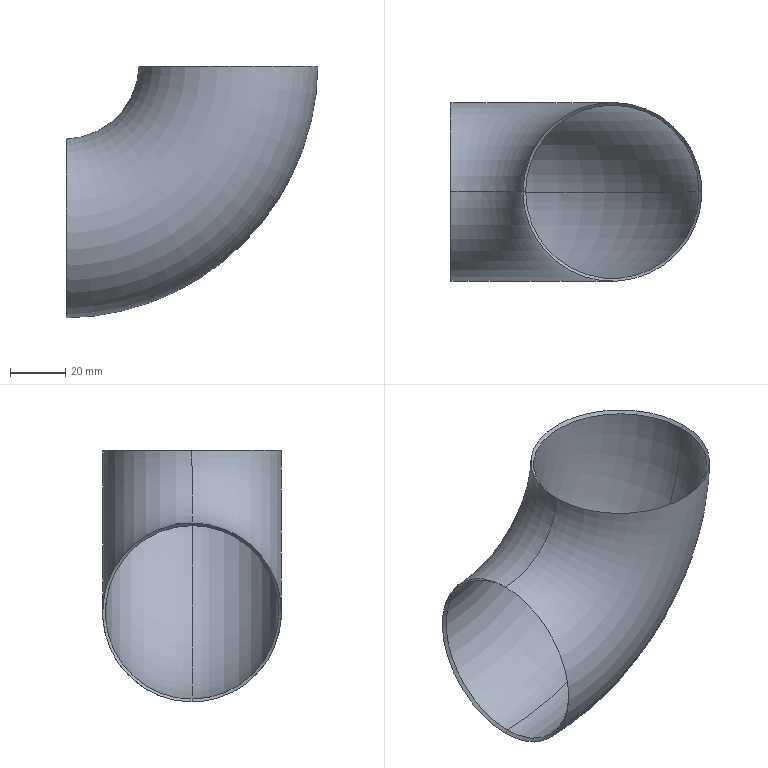Part | SolidWorks | features Chamfer 1, Revolution 1 | 1 solid | 8 faces | box 91.534 x 65 x 91.534 mm | volume 19075 mm3 | spline 4 | torus 4